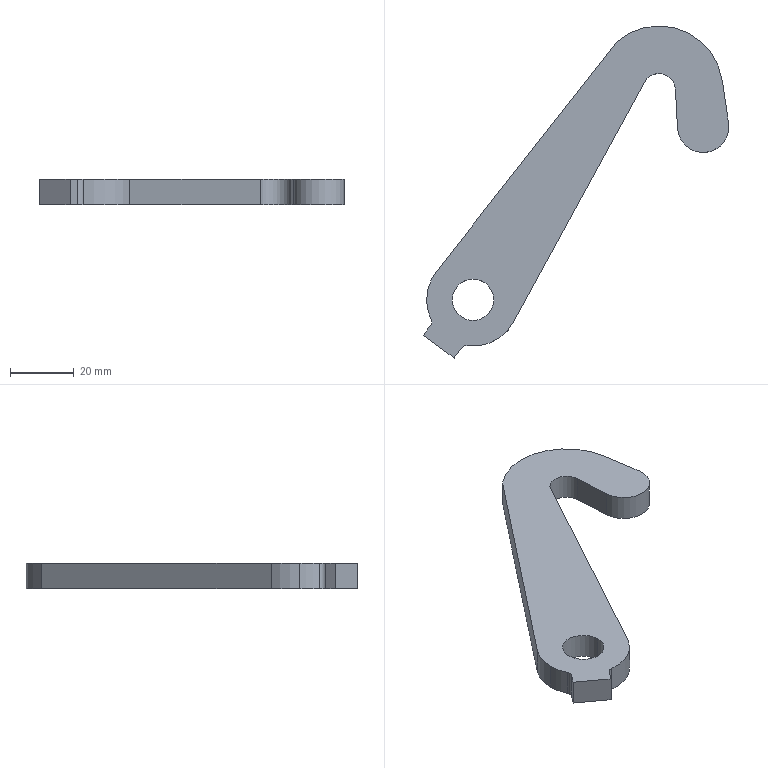Part | SolidWorks | features Extrusion 1, Fillet 1 | 1 solid | 19 faces | box 95.852 x 104.113 x 8 mm | volume 23315 mm3 | cylinder 10 | plane 9 | commonest cylinder face diameters 29.053 x3 4 x2 13 x2 10.359 x1 16.117 x1 40.167 x1
STEP:
#1=CARTESIAN_POINT('',(-12.64,-1.662,4.));
#2=VERTEX_POINT('',#1);
#3=CARTESIAN_POINT('',(0.3605,-1.662,4.));
#4=VERTEX_POINT('',#3);
#5=CARTESIAN_POINT('',(-6.14,-1.662,4.));
#6=DIRECTION('',(0.,0.,1.));
#7=DIRECTION('',(1.,0.,0.));
#8=AXIS2_PLACEMENT_3D('',#5,#6,#7);
#9=CIRCLE('',#8,6.5);
#10=EDGE_CURVE('',#2,#4,#9,.T.);
#11=ORIENTED_EDGE('',*,*,#10,.T.);
#12=CARTESIAN_POINT('',(0.3605,-1.662,-4.));
#13=VERTEX_POINT('',#12);
#14=CARTESIAN_POINT('',(0.3605,-1.662,4.));
#15=DIRECTION('',(0.,0.,-1.));
#16=VECTOR('',#15,1000.);
#17=LINE('',#14,#16);
#18=EDGE_CURVE('',#4,#13,#17,.T.);
#19=ORIENTED_EDGE('',*,*,#18,.T.);
#20=CARTESIAN_POINT('',(-12.64,-1.662,-4.));
#21=VERTEX_POINT('',#20);
#22=CARTESIAN_POINT('',(-6.14,-1.662,-4.));
#23=DIRECTION('',(0.,0.,1.));
#24=DIRECTION('',(1.,0.,0.));
#25=AXIS2_PLACEMENT_3D('',#22,#23,#24);
#26=CIRCLE('',#25,6.5);
#27=EDGE_CURVE('',#21,#13,#26,.T.);
#28=ORIENTED_EDGE('',*,*,#27,.F.);
#29=CARTESIAN_POINT('',(-12.64,-1.662,4.));
#30=DIRECTION('',(0.,0.,-1.));
#31=VECTOR('',#30,1000.);
#32=LINE('',#29,#31);
#33=EDGE_CURVE('',#2,#21,#32,.T.);
#34=ORIENTED_EDGE('',*,*,#33,.F.);
#35=EDGE_LOOP('',(#11,#19,#28,#34));
#36=FACE_OUTER_BOUND('',#35,.T.);
#37=CARTESIAN_POINT('',(-6.14,-1.662,4.));
#38=DIRECTION('',(0.,0.,-1.));
#39=DIRECTION('',(-1.,0.,0.));
#40=AXIS2_PLACEMENT_3D('',#37,#38,#39);
#41=CYLINDRICAL_SURFACE('',#40,6.5);
#42=ADVANCED_FACE('',(#36),#41,.F.);
#43=CARTESIAN_POINT('',(-20.666,-1.662,4.));
#44=VERTEX_POINT('',#43);
#45=CARTESIAN_POINT('',(-19.326,-7.756,4.));
#46=VERTEX_POINT('',#45);
#47=CARTESIAN_POINT('',(-6.14,-1.662,4.));
#48=DIRECTION('',(0.,0.,1.));
#49=DIRECTION('',(1.,0.,0.));
#50=AXIS2_PLACEMENT_3D('',#47,#48,#49);
#51=CIRCLE('',#50,14.527);
#52=EDGE_CURVE('',#44,#46,#51,.T.);
#53=ORIENTED_EDGE('',*,*,#52,.F.);
#54=CARTESIAN_POINT('',(-20.666,-1.662,-4.));
#55=VERTEX_POINT('',#54);
#56=CARTESIAN_POINT('',(-20.666,-1.662,4.));
#57=DIRECTION('',(0.,0.,-1.));
#58=VECTOR('',#57,1000.);
#59=LINE('',#56,#58);
#60=EDGE_CURVE('',#44,#55,#59,.T.);
#61=ORIENTED_EDGE('',*,*,#60,.T.);
#62=CARTESIAN_POINT('',(-19.326,-7.756,-4.));
#63=VERTEX_POINT('',#62);
#64=CARTESIAN_POINT('',(-6.14,-1.662,-4.));
#65=DIRECTION('',(0.,0.,1.));
#66=DIRECTION('',(1.,0.,0.));
#67=AXIS2_PLACEMENT_3D('',#64,#65,#66);
#68=CIRCLE('',#67,14.527);
#69=EDGE_CURVE('',#55,#63,#68,.T.);
#70=ORIENTED_EDGE('',*,*,#69,.T.);
#71=CARTESIAN_POINT('',(-19.326,-7.756,4.));
#72=DIRECTION('',(0.,0.,1.));
#73=VECTOR('',#72,1000.);
#74=LINE('',#71,#73);
#75=EDGE_CURVE('',#63,#46,#74,.T.);
#76=ORIENTED_EDGE('',*,*,#75,.T.);
#77=EDGE_LOOP('',(#53,#61,#70,#76));
#78=FACE_OUTER_BOUND('',#77,.T.);
#79=CARTESIAN_POINT('',(-6.14,-1.662,4.));
#80=DIRECTION('',(0.,0.,-1.));
#81=DIRECTION('',(-1.,0.,0.));
#82=AXIS2_PLACEMENT_3D('',#79,#80,#81);
#83=CYLINDRICAL_SURFACE('',#82,14.527);
#84=ADVANCED_FACE('',(#78),#83,.T.);
#85=CARTESIAN_POINT('',(-21.756,-12.817,4.));
#86=VERTEX_POINT('',#85);
#87=CARTESIAN_POINT('',(-12.078,-19.911,4.));
#88=VERTEX_POINT('',#87);
#89=CARTESIAN_POINT('',(-21.756,-12.817,4.));
#90=DIRECTION('',(0.8065,-0.5912,0.));
#91=VECTOR('',#90,1000.);
#92=LINE('',#89,#91);
#93=EDGE_CURVE('',#86,#88,#92,.T.);
#94=ORIENTED_EDGE('',*,*,#93,.T.);
#95=CARTESIAN_POINT('',(-9.85,-16.872,4.));
#96=VERTEX_POINT('',#95);
#97=CARTESIAN_POINT('',(-12.078,-19.911,4.));
#98=DIRECTION('',(0.5912,0.8065,0.));
#99=VECTOR('',#98,1000.);
#100=LINE('',#97,#99);
#101=EDGE_CURVE('',#88,#96,#100,.T.);
#102=ORIENTED_EDGE('',*,*,#101,.T.);
#103=CARTESIAN_POINT('',(-7.983,-16.071,4.));
#104=VERTEX_POINT('',#103);
#105=CARTESIAN_POINT('',(-8.237,-18.055,4.));
#106=DIRECTION('',(0.,0.,-1.));
#107=DIRECTION('',(1.,0.,0.));
#108=AXIS2_PLACEMENT_3D('',#105,#106,#107);
#109=CIRCLE('',#108,2.);
#110=EDGE_CURVE('',#96,#104,#109,.T.);
#111=ORIENTED_EDGE('',*,*,#110,.T.);
#112=CARTESIAN_POINT('',(6.615,-8.614,4.));
#113=VERTEX_POINT('',#112);
#114=CARTESIAN_POINT('',(-6.14,-1.662,4.));
#115=DIRECTION('',(0.,0.,1.));
#116=DIRECTION('',(1.,0.,0.));
#117=AXIS2_PLACEMENT_3D('',#114,#115,#116);
#118=CIRCLE('',#117,14.527);
#119=EDGE_CURVE('',#104,#113,#118,.T.);
#120=ORIENTED_EDGE('',*,*,#119,.T.);
#121=CARTESIAN_POINT('',(47.613,66.597,4.));
#122=VERTEX_POINT('',#121);
#123=CARTESIAN_POINT('',(47.613,66.597,4.));
#124=DIRECTION('',(0.4786,0.878,0.));
#125=VECTOR('',#124,1000.);
#126=LINE('',#123,#125);
#127=EDGE_CURVE('',#113,#122,#126,.T.);
#128=ORIENTED_EDGE('',*,*,#127,.T.);
#129=CARTESIAN_POINT('',(57.333,64.395,4.));
#130=VERTEX_POINT('',#129);
#131=CARTESIAN_POINT('',(52.161,64.118,4.));
#132=DIRECTION('',(0.,0.,-1.));
#133=DIRECTION('',(1.,0.,0.));
#134=AXIS2_PLACEMENT_3D('',#131,#132,#133);
#135=CIRCLE('',#134,5.18);
#136=EDGE_CURVE('',#122,#130,#135,.T.);
#137=ORIENTED_EDGE('',*,*,#136,.T.);
#138=CARTESIAN_POINT('',(57.991,52.141,4.));
#139=VERTEX_POINT('',#138);
#140=CARTESIAN_POINT('',(57.991,52.141,4.));
#141=DIRECTION('',(0.05357,-0.9986,0.));
#142=VECTOR('',#141,1000.);
#143=LINE('',#140,#142);
#144=EDGE_CURVE('',#130,#139,#143,.T.);
#145=ORIENTED_EDGE('',*,*,#144,.T.);
#146=CARTESIAN_POINT('',(74.008,53.759,4.));
#147=VERTEX_POINT('',#146);
#148=CARTESIAN_POINT('',(66.037,52.573,4.));
#149=DIRECTION('',(0.,0.,1.));
#150=DIRECTION('',(1.,0.,0.));
#151=AXIS2_PLACEMENT_3D('',#148,#149,#150);
#152=CIRCLE('',#151,8.058);
#153=EDGE_CURVE('',#139,#147,#152,.T.);
#154=ORIENTED_EDGE('',*,*,#153,.T.);
#155=CARTESIAN_POINT('',(72.026,67.075,4.));
#156=VERTEX_POINT('',#155);
#157=CARTESIAN_POINT('',(74.008,53.759,4.));
#158=DIRECTION('',(-0.1472,0.9891,0.));
#159=VECTOR('',#158,1000.);
#160=LINE('',#157,#159);
#161=EDGE_CURVE('',#147,#156,#160,.T.);
#162=ORIENTED_EDGE('',*,*,#161,.T.);
#163=CARTESIAN_POINT('',(39.076,79.354,4.));
#164=VERTEX_POINT('',#163);
#165=CARTESIAN_POINT('',(52.161,64.118,4.));
#166=DIRECTION('',(0.,0.,1.));
#167=DIRECTION('',(1.,0.,0.));
#168=AXIS2_PLACEMENT_3D('',#165,#166,#167);
#169=CIRCLE('',#168,20.084);
#170=EDGE_CURVE('',#156,#164,#169,.T.);
#171=ORIENTED_EDGE('',*,*,#170,.T.);
#172=CARTESIAN_POINT('',(-17.559,7.317,4.));
#173=VERTEX_POINT('',#172);
#174=CARTESIAN_POINT('',(39.076,79.354,4.));
#175=DIRECTION('',(-0.6181,-0.7861,0.));
#176=VECTOR('',#175,1000.);
#177=LINE('',#174,#176);
#178=EDGE_CURVE('',#164,#173,#177,.T.);
#179=ORIENTED_EDGE('',*,*,#178,.T.);
#180=CARTESIAN_POINT('',(-6.14,-1.662,4.));
#181=DIRECTION('',(0.,0.,1.));
#182=DIRECTION('',(1.,0.,0.));
#183=AXIS2_PLACEMENT_3D('',#180,#181,#182);
#184=CIRCLE('',#183,14.527);
#185=EDGE_CURVE('',#173,#44,#184,.T.);
#186=ORIENTED_EDGE('',*,*,#185,.T.);
#187=ORIENTED_EDGE('',*,*,#52,.T.);
#188=CARTESIAN_POINT('',(-19.528,-9.778,4.));
#189=VERTEX_POINT('',#188);
#190=CARTESIAN_POINT('',(-21.141,-8.595,4.));
#191=DIRECTION('',(0.,0.,-1.));
#192=DIRECTION('',(1.,0.,0.));
#193=AXIS2_PLACEMENT_3D('',#190,#191,#192);
#194=CIRCLE('',#193,2.);
#195=EDGE_CURVE('',#46,#189,#194,.T.);
#196=ORIENTED_EDGE('',*,*,#195,.T.);
#197=CARTESIAN_POINT('',(-18.8,-8.784,4.));
#198=DIRECTION('',(-0.5912,-0.8065,0.));
#199=VECTOR('',#198,1000.);
#200=LINE('',#197,#199);
#201=EDGE_CURVE('',#189,#86,#200,.T.);
#202=ORIENTED_EDGE('',*,*,#201,.T.);
#203=EDGE_LOOP('',(#94,#102,#111,#120,#128,#137,#145,#154,#162,#171,#179,#186,#187,#196,#202));
#204=FACE_OUTER_BOUND('',#203,.T.);
#205=ORIENTED_EDGE('',*,*,#10,.F.);
#206=CARTESIAN_POINT('',(-6.14,-1.662,4.));
#207=DIRECTION('',(0.,0.,1.));
#208=DIRECTION('',(1.,0.,0.));
#209=AXIS2_PLACEMENT_3D('',#206,#207,#208);
#210=CIRCLE('',#209,6.5);
#211=EDGE_CURVE('',#4,#2,#210,.T.);
#212=ORIENTED_EDGE('',*,*,#211,.F.);
#213=EDGE_LOOP('',(#205,#212));
#214=FACE_BOUND('',#213,.T.);
#215=CARTESIAN_POINT('',(-6.14,-1.662,4.));
#216=DIRECTION('',(0.,0.,1.));
#217=DIRECTION('',(1.,0.,0.));
#218=AXIS2_PLACEMENT_3D('',#215,#216,#217);
#219=PLANE('',#218);
#220=ADVANCED_FACE('',(#204,#214),#219,.T.);
#221=CARTESIAN_POINT('',(-21.756,-12.817,-4.));
#222=VERTEX_POINT('',#221);
#223=CARTESIAN_POINT('',(-12.078,-19.911,-4.));
#224=VERTEX_POINT('',#223);
#225=CARTESIAN_POINT('',(-21.756,-12.817,-4.));
#226=DIRECTION('',(0.8065,-0.5912,0.));
#227=VECTOR('',#226,1000.);
#228=LINE('',#225,#227);
#229=EDGE_CURVE('',#222,#224,#228,.T.);
#230=ORIENTED_EDGE('',*,*,#229,.F.);
#231=CARTESIAN_POINT('',(-19.528,-9.778,-4.));
#232=VERTEX_POINT('',#231);
#233=CARTESIAN_POINT('',(-18.8,-8.784,-4.));
#234=DIRECTION('',(-0.5912,-0.8065,0.));
#235=VECTOR('',#234,1000.);
#236=LINE('',#233,#235);
#237=EDGE_CURVE('',#232,#222,#236,.T.);
#238=ORIENTED_EDGE('',*,*,#237,.F.);
#239=CARTESIAN_POINT('',(-21.141,-8.595,-4.));
#240=DIRECTION('',(0.,0.,1.));
#241=DIRECTION('',(1.,0.,0.));
#242=AXIS2_PLACEMENT_3D('',#239,#240,#241);
#243=CIRCLE('',#242,2.);
#244=EDGE_CURVE('',#232,#63,#243,.T.);
#245=ORIENTED_EDGE('',*,*,#244,.T.);
#246=ORIENTED_EDGE('',*,*,#69,.F.);
#247=CARTESIAN_POINT('',(-17.559,7.317,-4.));
#248=VERTEX_POINT('',#247);
#249=CARTESIAN_POINT('',(-6.14,-1.662,-4.));
#250=DIRECTION('',(0.,0.,1.));
#251=DIRECTION('',(1.,0.,0.));
#252=AXIS2_PLACEMENT_3D('',#249,#250,#251);
#253=CIRCLE('',#252,14.527);
#254=EDGE_CURVE('',#248,#55,#253,.T.);
#255=ORIENTED_EDGE('',*,*,#254,.F.);
#256=CARTESIAN_POINT('',(39.076,79.354,-4.));
#257=VERTEX_POINT('',#256);
#258=CARTESIAN_POINT('',(39.076,79.354,-4.));
#259=DIRECTION('',(-0.6181,-0.7861,0.));
#260=VECTOR('',#259,1000.);
#261=LINE('',#258,#260);
#262=EDGE_CURVE('',#257,#248,#261,.T.);
#263=ORIENTED_EDGE('',*,*,#262,.F.);
#264=CARTESIAN_POINT('',(72.026,67.075,-4.));
#265=VERTEX_POINT('',#264);
#266=CARTESIAN_POINT('',(52.161,64.118,-4.));
#267=DIRECTION('',(0.,0.,1.));
#268=DIRECTION('',(1.,0.,0.));
#269=AXIS2_PLACEMENT_3D('',#266,#267,#268);
#270=CIRCLE('',#269,20.084);
#271=EDGE_CURVE('',#265,#257,#270,.T.);
#272=ORIENTED_EDGE('',*,*,#271,.F.);
#273=CARTESIAN_POINT('',(74.008,53.759,-4.));
#274=VERTEX_POINT('',#273);
#275=CARTESIAN_POINT('',(74.008,53.759,-4.));
#276=DIRECTION('',(-0.1472,0.9891,0.));
#277=VECTOR('',#276,1000.);
#278=LINE('',#275,#277);
#279=EDGE_CURVE('',#274,#265,#278,.T.);
#280=ORIENTED_EDGE('',*,*,#279,.F.);
#281=CARTESIAN_POINT('',(57.991,52.141,-4.));
#282=VERTEX_POINT('',#281);
#283=CARTESIAN_POINT('',(66.037,52.573,-4.));
#284=DIRECTION('',(0.,0.,1.));
#285=DIRECTION('',(1.,0.,0.));
#286=AXIS2_PLACEMENT_3D('',#283,#284,#285);
#287=CIRCLE('',#286,8.058);
#288=EDGE_CURVE('',#282,#274,#287,.T.);
#289=ORIENTED_EDGE('',*,*,#288,.F.);
#290=CARTESIAN_POINT('',(57.333,64.395,-4.));
#291=VERTEX_POINT('',#290);
#292=CARTESIAN_POINT('',(57.991,52.141,-4.));
#293=DIRECTION('',(0.05357,-0.9986,0.));
#294=VECTOR('',#293,1000.);
#295=LINE('',#292,#294);
#296=EDGE_CURVE('',#291,#282,#295,.T.);
#297=ORIENTED_EDGE('',*,*,#296,.F.);
#298=CARTESIAN_POINT('',(47.613,66.597,-4.));
#299=VERTEX_POINT('',#298);
#300=CARTESIAN_POINT('',(52.161,64.118,-4.));
#301=DIRECTION('',(0.,0.,-1.));
#302=DIRECTION('',(1.,0.,0.));
#303=AXIS2_PLACEMENT_3D('',#300,#301,#302);
#304=CIRCLE('',#303,5.18);
#305=EDGE_CURVE('',#299,#291,#304,.T.);
#306=ORIENTED_EDGE('',*,*,#305,.F.);
#307=CARTESIAN_POINT('',(6.615,-8.614,-4.));
#308=VERTEX_POINT('',#307);
#309=CARTESIAN_POINT('',(47.613,66.597,-4.));
#310=DIRECTION('',(0.4786,0.878,0.));
#311=VECTOR('',#310,1000.);
#312=LINE('',#309,#311);
#313=EDGE_CURVE('',#308,#299,#312,.T.);
#314=ORIENTED_EDGE('',*,*,#313,.F.);
#315=CARTESIAN_POINT('',(-7.983,-16.071,-4.));
#316=VERTEX_POINT('',#315);
#317=CARTESIAN_POINT('',(-6.14,-1.662,-4.));
#318=DIRECTION('',(0.,0.,1.));
#319=DIRECTION('',(1.,0.,0.));
#320=AXIS2_PLACEMENT_3D('',#317,#318,#319);
#321=CIRCLE('',#320,14.527);
#322=EDGE_CURVE('',#316,#308,#321,.T.);
#323=ORIENTED_EDGE('',*,*,#322,.F.);
#324=CARTESIAN_POINT('',(-9.85,-16.872,-4.));
#325=VERTEX_POINT('',#324);
#326=CARTESIAN_POINT('',(-8.237,-18.055,-4.));
#327=DIRECTION('',(0.,0.,1.));
#328=DIRECTION('',(1.,0.,0.));
#329=AXIS2_PLACEMENT_3D('',#326,#327,#328);
#330=CIRCLE('',#329,2.);
#331=EDGE_CURVE('',#316,#325,#330,.T.);
#332=ORIENTED_EDGE('',*,*,#331,.T.);
#333=CARTESIAN_POINT('',(-12.078,-19.911,-4.));
#334=DIRECTION('',(0.5912,0.8065,0.));
#335=VECTOR('',#334,1000.);
#336=LINE('',#333,#335);
#337=EDGE_CURVE('',#224,#325,#336,.T.);
#338=ORIENTED_EDGE('',*,*,#337,.F.);
#339=EDGE_LOOP('',(#230,#238,#245,#246,#255,#263,#272,#280,#289,#297,#306,#314,#323,#332,#338));
#340=FACE_OUTER_BOUND('',#339,.T.);
#341=ORIENTED_EDGE('',*,*,#27,.T.);
#342=CARTESIAN_POINT('',(-6.14,-1.662,-4.));
#343=DIRECTION('',(0.,0.,1.));
#344=DIRECTION('',(1.,0.,0.));
#345=AXIS2_PLACEMENT_3D('',#342,#343,#344);
#346=CIRCLE('',#345,6.5);
#347=EDGE_CURVE('',#13,#21,#346,.T.);
#348=ORIENTED_EDGE('',*,*,#347,.T.);
#349=EDGE_LOOP('',(#341,#348));
#350=FACE_BOUND('',#349,.T.);
#351=CARTESIAN_POINT('',(-6.14,-1.662,-4.));
#352=DIRECTION('',(0.,0.,1.));
#353=DIRECTION('',(1.,0.,0.));
#354=AXIS2_PLACEMENT_3D('',#351,#352,#353);
#355=PLANE('',#354);
#356=ADVANCED_FACE('',(#340,#350),#355,.F.);
#357=ORIENTED_EDGE('',*,*,#229,.T.);
#358=CARTESIAN_POINT('',(-12.078,-19.911,4.));
#359=DIRECTION('',(0.,0.,-1.));
#360=VECTOR('',#359,1000.);
#361=LINE('',#358,#360);
#362=EDGE_CURVE('',#88,#224,#361,.T.);
#363=ORIENTED_EDGE('',*,*,#362,.F.);
#364=ORIENTED_EDGE('',*,*,#93,.F.);
#365=CARTESIAN_POINT('',(-21.756,-12.817,4.));
#366=DIRECTION('',(0.,0.,-1.));
#367=VECTOR('',#366,1000.);
#368=LINE('',#365,#367);
#369=EDGE_CURVE('',#86,#222,#368,.T.);
#370=ORIENTED_EDGE('',*,*,#369,.T.);
#371=EDGE_LOOP('',(#357,#363,#364,#370));
#372=FACE_OUTER_BOUND('',#371,.T.);
#373=CARTESIAN_POINT('',(-21.756,-12.817,4.));
#374=DIRECTION('',(0.5912,0.8065,0.));
#375=DIRECTION('',(-0.8065,0.5912,0.));
#376=AXIS2_PLACEMENT_3D('',#373,#374,#375);
#377=PLANE('',#376);
#378=ADVANCED_FACE('',(#372),#377,.F.);
#379=ORIENTED_EDGE('',*,*,#337,.T.);
#380=CARTESIAN_POINT('',(-9.85,-16.872,4.));
#381=DIRECTION('',(0.,0.,1.));
#382=VECTOR('',#381,1000.);
#383=LINE('',#380,#382);
#384=EDGE_CURVE('',#325,#96,#383,.T.);
#385=ORIENTED_EDGE('',*,*,#384,.T.);
#386=ORIENTED_EDGE('',*,*,#101,.F.);
#387=ORIENTED_EDGE('',*,*,#362,.T.);
#388=EDGE_LOOP('',(#379,#385,#386,#387));
#389=FACE_OUTER_BOUND('',#388,.T.);
#390=CARTESIAN_POINT('',(-12.078,-19.911,4.));
#391=DIRECTION('',(-0.8065,0.5912,0.));
#392=DIRECTION('',(-0.5912,-0.8065,0.));
#393=AXIS2_PLACEMENT_3D('',#390,#391,#392);
#394=PLANE('',#393);
#395=ADVANCED_FACE('',(#389),#394,.F.);
#396=ORIENTED_EDGE('',*,*,#119,.F.);
#397=CARTESIAN_POINT('',(-7.983,-16.071,4.));
#398=DIRECTION('',(0.,0.,-1.));
#399=VECTOR('',#398,1000.);
#400=LINE('',#397,#399);
#401=EDGE_CURVE('',#104,#316,#400,.T.);
#402=ORIENTED_EDGE('',*,*,#401,.T.);
#403=ORIENTED_EDGE('',*,*,#322,.T.);
#404=CARTESIAN_POINT('',(6.615,-8.614,4.));
#405=DIRECTION('',(0.,0.,-1.));
#406=VECTOR('',#405,1000.);
#407=LINE('',#404,#406);
#408=EDGE_CURVE('',#113,#308,#407,.T.);
#409=ORIENTED_EDGE('',*,*,#408,.F.);
#410=EDGE_LOOP('',(#396,#402,#403,#409));
#411=FACE_OUTER_BOUND('',#410,.T.);
#412=CARTESIAN_POINT('',(-6.14,-1.662,4.));
#413=DIRECTION('',(0.,0.,-1.));
#414=DIRECTION('',(-1.,0.,0.));
#415=AXIS2_PLACEMENT_3D('',#412,#413,#414);
#416=CYLINDRICAL_SURFACE('',#415,14.527);
#417=ADVANCED_FACE('',(#411),#416,.T.);
#418=ORIENTED_EDGE('',*,*,#313,.T.);
#419=CARTESIAN_POINT('',(47.613,66.597,4.));
#420=DIRECTION('',(0.,0.,-1.));
#421=VECTOR('',#420,1000.);
#422=LINE('',#419,#421);
#423=EDGE_CURVE('',#122,#299,#422,.T.);
#424=ORIENTED_EDGE('',*,*,#423,.F.);
#425=ORIENTED_EDGE('',*,*,#127,.F.);
#426=ORIENTED_EDGE('',*,*,#408,.T.);
#427=EDGE_LOOP('',(#418,#424,#425,#426));
#428=FACE_OUTER_BOUND('',#427,.T.);
#429=CARTESIAN_POINT('',(47.613,66.597,4.));
#430=DIRECTION('',(-0.878,0.4786,0.));
#431=DIRECTION('',(-0.4786,-0.878,0.));
#432=AXIS2_PLACEMENT_3D('',#429,#430,#431);
#433=PLANE('',#432);
#434=ADVANCED_FACE('',(#428),#433,.F.);
#435=ORIENTED_EDGE('',*,*,#305,.T.);
#436=CARTESIAN_POINT('',(57.333,64.395,4.));
#437=DIRECTION('',(0.,0.,-1.));
#438=VECTOR('',#437,1000.);
#439=LINE('',#436,#438);
#440=EDGE_CURVE('',#130,#291,#439,.T.);
#441=ORIENTED_EDGE('',*,*,#440,.F.);
#442=ORIENTED_EDGE('',*,*,#136,.F.);
#443=ORIENTED_EDGE('',*,*,#423,.T.);
#444=EDGE_LOOP('',(#435,#441,#442,#443));
#445=FACE_OUTER_BOUND('',#444,.T.);
#446=CARTESIAN_POINT('',(52.161,64.118,4.));
#447=DIRECTION('',(0.,0.,-1.));
#448=DIRECTION('',(-1.,0.,0.));
#449=AXIS2_PLACEMENT_3D('',#446,#447,#448);
#450=CYLINDRICAL_SURFACE('',#449,5.18);
#451=ADVANCED_FACE('',(#445),#450,.F.);
#452=ORIENTED_EDGE('',*,*,#296,.T.);
#453=CARTESIAN_POINT('',(57.991,52.141,4.));
#454=DIRECTION('',(0.,0.,-1.));
#455=VECTOR('',#454,1000.);
#456=LINE('',#453,#455);
#457=EDGE_CURVE('',#139,#282,#456,.T.);
#458=ORIENTED_EDGE('',*,*,#457,.F.);
#459=ORIENTED_EDGE('',*,*,#144,.F.);
#460=ORIENTED_EDGE('',*,*,#440,.T.);
#461=EDGE_LOOP('',(#452,#458,#459,#460));
#462=FACE_OUTER_BOUND('',#461,.T.);
#463=CARTESIAN_POINT('',(57.991,52.141,4.));
#464=DIRECTION('',(0.9986,0.05357,0.));
#465=DIRECTION('',(-0.05357,0.9986,0.));
#466=AXIS2_PLACEMENT_3D('',#463,#464,#465);
#467=PLANE('',#466);
#468=ADVANCED_FACE('',(#462),#467,.F.);
#469=ORIENTED_EDGE('',*,*,#288,.T.);
#470=CARTESIAN_POINT('',(74.008,53.759,4.));
#471=DIRECTION('',(0.,0.,-1.));
#472=VECTOR('',#471,1000.);
#473=LINE('',#470,#472);
#474=EDGE_CURVE('',#147,#274,#473,.T.);
#475=ORIENTED_EDGE('',*,*,#474,.F.);
#476=ORIENTED_EDGE('',*,*,#153,.F.);
#477=ORIENTED_EDGE('',*,*,#457,.T.);
#478=EDGE_LOOP('',(#469,#475,#476,#477));
#479=FACE_OUTER_BOUND('',#478,.T.);
#480=CARTESIAN_POINT('',(66.037,52.573,4.));
#481=DIRECTION('',(0.,0.,-1.));
#482=DIRECTION('',(-1.,0.,0.));
#483=AXIS2_PLACEMENT_3D('',#480,#481,#482);
#484=CYLINDRICAL_SURFACE('',#483,8.058);
#485=ADVANCED_FACE('',(#479),#484,.T.);
#486=ORIENTED_EDGE('',*,*,#279,.T.);
#487=CARTESIAN_POINT('',(72.026,67.075,4.));
#488=DIRECTION('',(0.,0.,-1.));
#489=VECTOR('',#488,1000.);
#490=LINE('',#487,#489);
#491=EDGE_CURVE('',#156,#265,#490,.T.);
#492=ORIENTED_EDGE('',*,*,#491,.F.);
#493=ORIENTED_EDGE('',*,*,#161,.F.);
#494=ORIENTED_EDGE('',*,*,#474,.T.);
#495=EDGE_LOOP('',(#486,#492,#493,#494));
#496=FACE_OUTER_BOUND('',#495,.T.);
#497=CARTESIAN_POINT('',(74.008,53.759,4.));
#498=DIRECTION('',(-0.9891,-0.1472,0.));
#499=DIRECTION('',(0.1472,-0.9891,0.));
#500=AXIS2_PLACEMENT_3D('',#497,#498,#499);
#501=PLANE('',#500);
#502=ADVANCED_FACE('',(#496),#501,.F.);
#503=ORIENTED_EDGE('',*,*,#271,.T.);
#504=CARTESIAN_POINT('',(39.076,79.354,4.));
#505=DIRECTION('',(0.,0.,-1.));
#506=VECTOR('',#505,1000.);
#507=LINE('',#504,#506);
#508=EDGE_CURVE('',#164,#257,#507,.T.);
#509=ORIENTED_EDGE('',*,*,#508,.F.);
#510=ORIENTED_EDGE('',*,*,#170,.F.);
#511=ORIENTED_EDGE('',*,*,#491,.T.);
#512=EDGE_LOOP('',(#503,#509,#510,#511));
#513=FACE_OUTER_BOUND('',#512,.T.);
#514=CARTESIAN_POINT('',(52.161,64.118,4.));
#515=DIRECTION('',(0.,0.,-1.));
#516=DIRECTION('',(-1.,0.,0.));
#517=AXIS2_PLACEMENT_3D('',#514,#515,#516);
#518=CYLINDRICAL_SURFACE('',#517,20.084);
#519=ADVANCED_FACE('',(#513),#518,.T.);
#520=ORIENTED_EDGE('',*,*,#262,.T.);
#521=CARTESIAN_POINT('',(-17.559,7.317,4.));
#522=DIRECTION('',(0.,0.,-1.));
#523=VECTOR('',#522,1000.);
#524=LINE('',#521,#523);
#525=EDGE_CURVE('',#173,#248,#524,.T.);
#526=ORIENTED_EDGE('',*,*,#525,.F.);
#527=ORIENTED_EDGE('',*,*,#178,.F.);
#528=ORIENTED_EDGE('',*,*,#508,.T.);
#529=EDGE_LOOP('',(#520,#526,#527,#528));
#530=FACE_OUTER_BOUND('',#529,.T.);
#531=CARTESIAN_POINT('',(39.076,79.354,4.));
#532=DIRECTION('',(0.7861,-0.6181,0.));
#533=DIRECTION('',(0.6181,0.7861,0.));
#534=AXIS2_PLACEMENT_3D('',#531,#532,#533);
#535=PLANE('',#534);
#536=ADVANCED_FACE('',(#530),#535,.F.);
#537=ORIENTED_EDGE('',*,*,#60,.F.);
#538=ORIENTED_EDGE('',*,*,#185,.F.);
#539=ORIENTED_EDGE('',*,*,#525,.T.);
#540=ORIENTED_EDGE('',*,*,#254,.T.);
#541=EDGE_LOOP('',(#537,#538,#539,#540));
#542=FACE_OUTER_BOUND('',#541,.T.);
#543=CARTESIAN_POINT('',(-6.14,-1.662,4.));
#544=DIRECTION('',(0.,0.,-1.));
#545=DIRECTION('',(-1.,0.,0.));
#546=AXIS2_PLACEMENT_3D('',#543,#544,#545);
#547=CYLINDRICAL_SURFACE('',#546,14.527);
#548=ADVANCED_FACE('',(#542),#547,.T.);
#549=ORIENTED_EDGE('',*,*,#201,.F.);
#550=CARTESIAN_POINT('',(-19.528,-9.778,-4.));
#551=DIRECTION('',(0.,0.,-1.));
#552=VECTOR('',#551,1000.);
#553=LINE('',#550,#552);
#554=EDGE_CURVE('',#189,#232,#553,.T.);
#555=ORIENTED_EDGE('',*,*,#554,.T.);
#556=ORIENTED_EDGE('',*,*,#237,.T.);
#557=ORIENTED_EDGE('',*,*,#369,.F.);
#558=EDGE_LOOP('',(#549,#555,#556,#557));
#559=FACE_OUTER_BOUND('',#558,.T.);
#560=CARTESIAN_POINT('',(-18.8,-8.784,4.));
#561=DIRECTION('',(0.8065,-0.5912,0.));
#562=DIRECTION('',(0.5912,0.8065,0.));
#563=AXIS2_PLACEMENT_3D('',#560,#561,#562);
#564=PLANE('',#563);
#565=ADVANCED_FACE('',(#559),#564,.F.);
#566=ORIENTED_EDGE('',*,*,#18,.F.);
#567=ORIENTED_EDGE('',*,*,#211,.T.);
#568=ORIENTED_EDGE('',*,*,#33,.T.);
#569=ORIENTED_EDGE('',*,*,#347,.F.);
#570=EDGE_LOOP('',(#566,#567,#568,#569));
#571=FACE_OUTER_BOUND('',#570,.T.);
#572=CARTESIAN_POINT('',(-6.14,-1.662,4.));
#573=DIRECTION('',(0.,0.,-1.));
#574=DIRECTION('',(-1.,0.,0.));
#575=AXIS2_PLACEMENT_3D('',#572,#573,#574);
#576=CYLINDRICAL_SURFACE('',#575,6.5);
#577=ADVANCED_FACE('',(#571),#576,.F.);
#578=ORIENTED_EDGE('',*,*,#110,.F.);
#579=ORIENTED_EDGE('',*,*,#384,.F.);
#580=ORIENTED_EDGE('',*,*,#331,.F.);
#581=ORIENTED_EDGE('',*,*,#401,.F.);
#582=EDGE_LOOP('',(#578,#579,#580,#581));
#583=FACE_OUTER_BOUND('',#582,.T.);
#584=CARTESIAN_POINT('',(-8.237,-18.055,4.));
#585=DIRECTION('',(0.,0.,-1.));
#586=DIRECTION('',(-1.,0.,0.));
#587=AXIS2_PLACEMENT_3D('',#584,#585,#586);
#588=CYLINDRICAL_SURFACE('',#587,2.);
#589=ADVANCED_FACE('',(#583),#588,.F.);
#590=ORIENTED_EDGE('',*,*,#195,.F.);
#591=ORIENTED_EDGE('',*,*,#75,.F.);
#592=ORIENTED_EDGE('',*,*,#244,.F.);
#593=ORIENTED_EDGE('',*,*,#554,.F.);
#594=EDGE_LOOP('',(#590,#591,#592,#593));
#595=FACE_OUTER_BOUND('',#594,.T.);
#596=CARTESIAN_POINT('',(-21.141,-8.595,4.));
#597=DIRECTION('',(0.,0.,-1.));
#598=DIRECTION('',(-1.,0.,0.));
#599=AXIS2_PLACEMENT_3D('',#596,#597,#598);
#600=CYLINDRICAL_SURFACE('',#599,2.);
#601=ADVANCED_FACE('',(#595),#600,.F.);
#602=CLOSED_SHELL('',(#42,#84,#220,#356,#378,#395,#417,#434,#451,#468,#485,#502,#519,#536,#548,#565,#577,#589,#601));
#603=MANIFOLD_SOLID_BREP('',#602);
#604=CARTESIAN_POINT('',(0.,0.,0.));
#605=DIRECTION('',(0.,0.,1.));
#606=DIRECTION('',(1.,0.,0.));
#607=AXIS2_PLACEMENT_3D('',#604,#605,#606);
#608=(LENGTH_UNIT()NAMED_UNIT(*)SI_UNIT(.MILLI.,.METRE.));
#609=UNCERTAINTY_MEASURE_WITH_UNIT(LENGTH_MEASURE(0.00001),#608,'','');
#610=(NAMED_UNIT(*)PLANE_ANGLE_UNIT()SI_UNIT($,.RADIAN.));
#611=(NAMED_UNIT(*)SI_UNIT($,.STERADIAN.)SOLID_ANGLE_UNIT());
#612=(GEOMETRIC_REPRESENTATION_CONTEXT(3)GLOBAL_UNCERTAINTY_ASSIGNED_CONTEXT((#609))GLOBAL_UNIT_ASSIGNED_CONTEXT((#608,#610,#611))REPRESENTATION_CONTEXT('',''));
#613=ADVANCED_BREP_SHAPE_REPRESENTATION('',(#603,#607),#612);